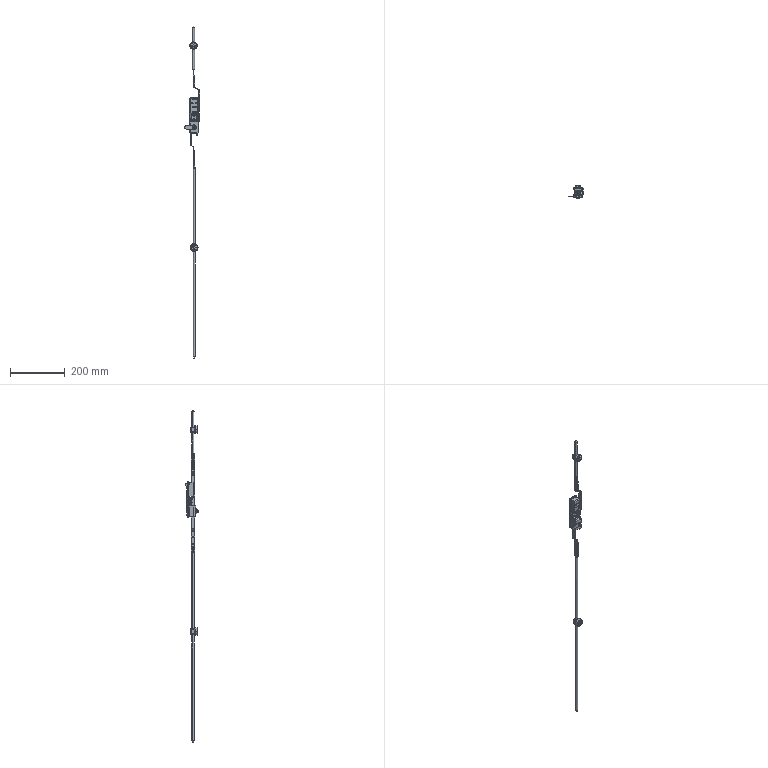Part | SolidWorks | 5 solids | 1056 faces | box 55.3 x 46.477 x 1208 mm | volume 150229 mm3 | cylinder 451 | plane 396 | spline 178 | cone 23 | torus 8 | commonest cylinder face diameters 1 x144 6.1 x70 0.8 x52 2 x26 16 x26 1.6 x24